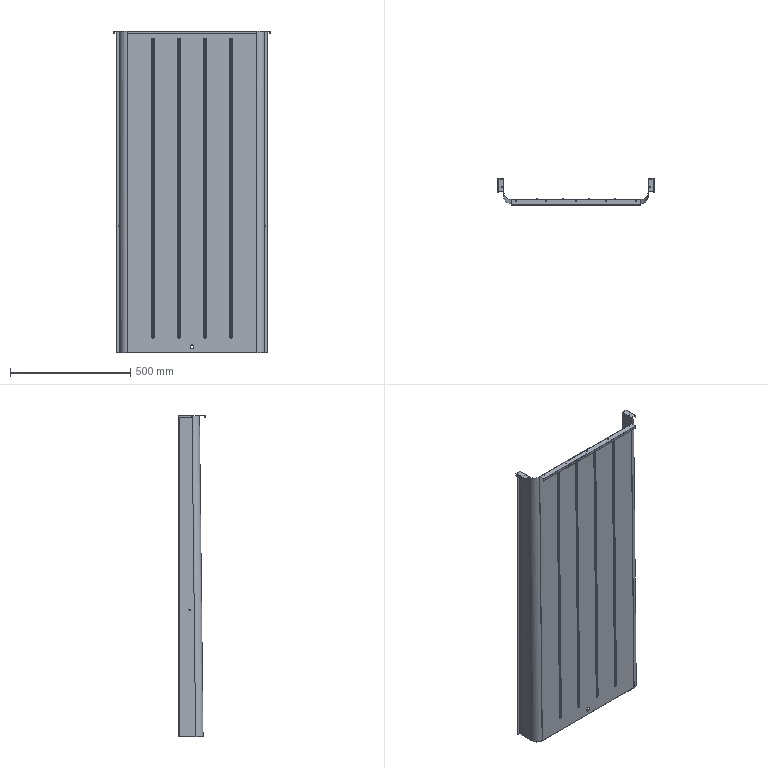Part | STEP file | HESS-408-70-15W-N-2-inner liner lower cover | 1 solid | 170 faces | box 650 x 110 x 1338 mm | volume 1081692 mm3 | cylinder 78 | plane 50 | spline 42 | commonest cylinder face diameters 3.5 x14 0.2 x8 0.4 x8 2.2 x8 2.4 x8 12 x8